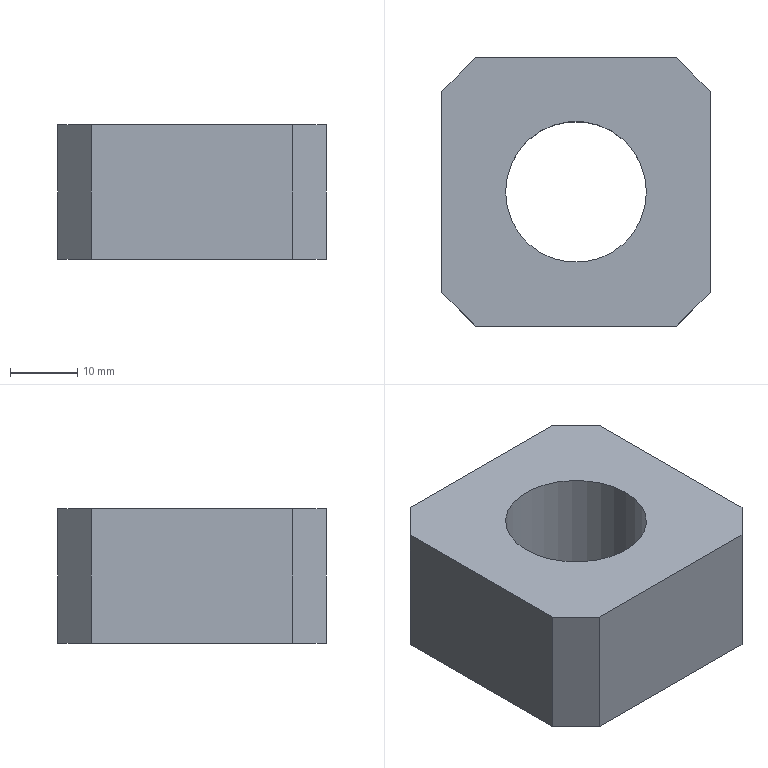NC program | NX | posted with a generic post | part box 40 x 40 x 20 mm
Whole program:
N10 G17 G21 G94 G90
(ADAPTIVE_MILLING_COPY_1 , TOOL : D10开粗)
N12 T05 M6
N14 G54
N16 G17 G0 G90 X-33.049 Y-20.536 S3500 M3
N18 G43 Z30. H5
N20 Z3.1
N22 G94 G1 X-32.899 Y-20.542 Z2.163 F1500.
N24 X-32.749 Y-20.549 Z1.792
N26 X-32.599 Y-20.555 Z1.52
N28 X-32.449 Y-20.561 Z1.3
N30 X-32.3 Y-20.568 Z1.116
N32 X-32.15 Y-20.574 Z0.958
N34 X-32. Y-20.581 Z0.82
N36 X-31.85 Y-20.587 Z0.7
N38 X-31.7 Y-20.593 Z0.595
N40 X-31.55 Y-20.6 Z0.502
N42 X-31.4 Y-20.606 Z0.421
N44 X-31.251 Y-20.613 Z0.35
N46 X-31.101 Y-20.619 Z0.29
N48 X-30.951 Y-20.625 Z0.238
N50 X-30.801 Y-20.632 Z0.195
N52 X-30.651 Y-20.638 Z0.161
N54 X-30.501 Y-20.645 Z0.134
N56 X-30.351 Y-20.651 Z0.115
N58 X-30.202 Y-20.657 Z0.104
N60 X-30.052 Y-20.664 Z0.1
N62 X-28.523 Y-20.729
N64 G3 X-27.505 Y-19.981 R1.01
N66 X-27.242 Y-16.948 R15.515
N68 X-27.2 Y-10.244 R592.762
N70 G1 X-27.198 Y20.693
N72 G2 X-24.571 Y25.413 R5.737
N74 X-20.324 Y26.917 R9.801
N76 X-14.522 Y27.19 R46.809
N78 G1 X-9.309 Y27.2
N80 X20.692 Y27.198
N82 G2 X25.369 Y24.633 R5.722
N84 X26.9 Y20.444 R9.633
N86 X27.187 Y14.906 R42.38
N88 G1 X27.2 Y9.281
N90 X27.198 Y-20.679
N92 G2 X24.594 Y-25.392 R5.737
N94 X20.28 Y-26.922 R9.807
N96 X14.44 Y-27.19 R47.799
N98 G1 X8.928 Y-27.2
N100 X-20.604 Y-27.199
N102 G2 X-25.345 Y-24.661 R5.722
N104 X-26.773 Y-20.525 R8.599
N106 X-26.912 Y-16.142 R43.012
N108 G1 X-26.9 Y-8.932
N110 X-26.899 Y19.193
N112 G2 X-23.364 Y25.142 R6.971
N114 X-18.636 Y26.621 R11.938
N116 X-12.533 Y26.888 R55.522
N118 G1 X-6.72 Y26.9
N120 X19.192 Y26.898
N122 G2 X25.165 Y23.325 R6.978
N124 X26.63 Y18.556 R12.069
N126 X26.888 Y12.64 R55.725
N128 G1 X26.899 Y7.278
N130 X26.898 Y-19.217
N132 G2 X23.336 Y-25.156 R6.98
N134 X18.604 Y-26.624 R12.015
N136 X12.35 Y-26.89 R57.25
N138 G1 X6.575 Y-26.9
N140 X-19.217 Y-26.898
N142 G2 X-25.194 Y-23.143 R6.82
N144 X-26.439 Y-18.463 R12.117
N146 X-26.598 Y-12.73 R71.518
N148 G1 X-26.6 Y-10.255
N150 X-26.598 Y17.808
N152 G2 X-22.197 Y24.971 R7.868
N154 X-17.27 Y26.331 R13.908
N156 X-10.941 Y26.588 R64.101
N158 G1 X-5.991 Y26.599
N160 X17.804 Y26.597
N162 G2 X24.955 Y22.227 R7.863
N164 X26.34 Y17.193 R13.966
N166 X26.592 Y10.113 R73.066
N168 G1 X26.599 Y5.988
N170 X26.598 Y-17.791
N172 G2 X22.197 Y-24.969 R7.872
N174 X17.31 Y-26.326 R13.869
N176 X10.718 Y-26.589 R65.387
N178 G1 X4.943 Y-26.599
N180 X-17.792 Y-26.598
N182 G2 X-24.818 Y-22.247 R7.64
N184 X-26.091 Y-17.376 R13.614
N186 X-26.294 Y-11.044 R72.736
N188 G1 X-26.3 Y-6.507
N190 X-26.298 Y16.567
N192 G2 X-24.928 Y21.595 R8.969
N194 X-20.056 Y25.221 R9.364
N196 X-14.753 Y26.151 R20.
N198 X-6.73 Y26.297 R146.883
N200 G1 X16.267 Y26.299
N202 G2 X20.613 Y25.476 R9.774
N204 X24.987 Y20.672 R8.891
N206 X26.109 Y15.335 R17.659
N208 X26.297 Y6.901 R121.733
N210 G1 X26.299 Y3.601
N212 X26.297 Y-16.555
N214 G2 X24.914 Y-21.615 R8.972
N216 X20.077 Y-25.212 R9.365
N218 X14.626 Y-26.158 R20.195
N220 X5.403 Y-26.298 R177.641
N222 G1 X-16.254 Y-26.299
N224 G2 X-20.559 Y-25.47 R9.497
N226 X-24.816 Y-20.672 R8.705
N228 X-25.844 Y-15.465 R17.595
N230 X-25.997 Y-8.193 R119.783
N232 G1 X-26. Y-4.48
N234 X-25.998 Y15.329
N236 G2 X-25.204 Y19.8 R10.961
N238 X-20.275 Y24.529 R9.234
N240 X-14.924 Y25.759 R17.439
N242 X-7.055 Y25.993 R95.576
N244 G1 X-2.105 Y25.999
N246 X15.254 Y25.998
N248 G2 X19.628 Y25.276 R11.231
N250 X24.518 Y20.302 R9.202
N252 X25.749 Y15.028 R17.246
N254 X25.994 Y6.972 R94.179
N256 G1 X25.999 Y2.435
N258 X25.997 Y-15.391
N260 G2 X25.163 Y-19.891 R10.767
N262 X20.219 Y-24.552 R9.27
N264 X14.939 Y-25.757 R17.515
N266 X6.845 Y-25.994 R97.367
N268 G1 X2.308 Y-25.999
N270 X-15.392 Y-25.997
N272 G2 X-19.916 Y-25.11 R10.327
N274 X-24.358 Y-20.239 R9.109
N276 X-25.504 Y-14.87 R17.702
N278 X-25.696 Y-7.074 R109.534
N280 G1 X-25.699 Y-2.949
N282 X-25.698 Y14.204
N284 G2 X-25.118 Y18.532 R13.216
N286 X-19.915 Y24.078 R9.477
N288 X-14.398 Y25.423 R17.467
N290 X-6.98 Y25.689 R83.266
N292 G1 X-1.205 Y25.698
N294 X14.242 Y25.697
N296 G2 X18.603 Y25.093 R13.026
N298 X24.065 Y19.942 R9.475
N300 X25.408 Y14.542 R17.238
N302 X25.689 Y6.937 R81.095
N304 G1 X25.698 Y1.162
N306 X25.697 Y-14.229
N308 G2 X25.096 Y-18.591 R13.073
N310 X19.967 Y-24.052 R9.468
N312 X14.344 Y-25.427 R17.479
N314 X6.964 Y-25.689 R84.191
N316 G1 X1.189 Y-25.698
N318 X-14.229 Y-25.697
N320 G2 X-18.514 Y-25.09 R12.561
N322 X-23.834 Y-20.017 R9.295
N324 X-25.148 Y-14.536 R17.186
N326 X-25.391 Y-7.155 R86.685
N328 G1 X-25.399 Y-1.792
N330 X-25.398 Y13.117
N332 G2 X-24.954 Y17.393 R16.031
N334 X-19.52 Y23.659 R9.748
N336 X-13.949 Y25.083 R17.521
N338 X-6.608 Y25.384 R75.983
N340 G1 X-0.008 Y25.398
N342 X13.154 Y25.397
N344 G2 X17.537 Y24.913 R15.59
N346 X23.632 Y19.576 R9.74
N348 X25.076 Y14.012 R17.369
N350 X25.387 Y6.146 R79.024
N352 G1 X25.398 Y-0.041
N354 X25.397 Y-13.142
N356 G2 X24.916 Y-17.525 R15.64
N358 X19.439 Y-23.695 R9.776
N360 X13.75 Y-25.104 R17.916
N362 X5.996 Y-25.388 R84.539
N364 G1 X0.221 Y-25.398
N366 X-13.104 Y-25.397
N368 G2 X-17.376 Y-24.928 R15.231
N370 X-23.41 Y-19.612 R9.58
N372 X-24.814 Y-13.999 R17.389
N374 X-25.089 Y-6.507 R81.982
N376 G1 X-25.099 Y-0.732
N378 X-25.098 Y12.067
N380 G2 X-24.727 Y16.428 R19.116
N382 X-19.044 Y23.294 R10.041
N384 X-13.405 Y24.758 R17.875
N386 X-6.066 Y25.081 R73.481
N388 G1 X0.947 Y25.098
N390 G2 X13.566 Y25.073 R883.653
N392 X18.614 Y23.948 R12.059
N394 X23.491 Y18.605 R10.333
N396 X24.816 Y12.854 R19.332
N398 X25.091 Y4.386 R97.895
N400 G1 X25.098 Y-0.976
N402 G2 X25.072 Y-13.591 R877.786
N404 X23.936 Y-18.636 R12.001
N406 X18.456 Y-23.552 R10.383
N408 X12.768 Y-24.824 R19.72
N410 X4.263 Y-25.091 R100.704
N412 G1 X-1.1 Y-25.098
N414 G2 X-13.516 Y-25.073 R869.408
N416 X-18.589 Y-23.888 R11.641
N418 X-23.333 Y-18.454 R10.277
N420 X-24.561 Y-12.678 R20.017
N422 X-24.791 Y-4.996 R102.276
N424 G1 X-24.799 Y0.367
N426 G2 X-24.766 Y12.966 R695.277
N428 X-23.623 Y18.088 R12.565
N430 X-18.063 Y23.168 R10.611
N432 X-12.2 Y24.508 R19.972
N434 X-3.47 Y24.79 R100.959
N436 G1 X1.892 Y24.798
N438 G2 X12.966 Y24.765 R584.678
N440 X18.19 Y23.571 R12.491
N442 X23.199 Y17.987 R10.652
N444 X24.523 Y12.044 R20.323
N446 X24.79 Y3.463 R103.915
N448 G1 X24.798 Y-1.899
N450 G2 X24.763 Y-13.029 R530.358
N452 X23.526 Y-18.278 R12.338
N454 X17.981 Y-23.201 R10.672
N456 X12.034 Y-24.523 R20.358
N458 X3.379 Y-24.791 R104.815
N460 G1 X-1.984 Y-24.798
N462 G2 X-12.954 Y-24.762 R509.573
N464 X-18.162 Y-23.504 R12.012
N466 X-22.959 Y-18.016 R10.553
N468 X-24.237 Y-12.176 R20.208
N470 X-24.49 Y-4.082 R101.04
N472 G1 X-24.498 Y1.28
N474 G2 X-24.462 Y12.291 R531.23
N476 X-23.338 Y17.496 R13.21
N478 X-17.629 Y22.809 R10.831
N480 X-11.734 Y24.185 R20.152
N482 X-3.68 Y24.485 R90.169
N484 G1 X2.507 Y24.497
N486 G2 X12.291 Y24.462 R456.381
N488 X17.428 Y23.369 R13.265
N490 X22.779 Y17.697 R10.805
N492 X24.196 Y11.621 R20.222
N494 X24.489 Y2.854 R99.947
N496 G1 X24.497 Y-2.508
N498 G2 X24.461 Y-12.316 R441.93
N500 X23.31 Y-17.553 R13.133
N502 X17.678 Y-22.786 R10.826
N504 X11.751 Y-24.182 R20.063
N506 X3.697 Y-24.485 R89.522
N508 G1 X-2.49 Y-24.497
N510 G2 X-12.241 Y-24.46 R419.199
N512 X-17.4 Y-23.305 R12.805
N514 X-22.545 Y-17.7 R10.717
N516 X-23.904 Y-11.798 R20.059
N518 X-24.186 Y-3.893 R91.732
N520 G1 X-24.198 Y2.295
N522 G2 X-24.16 Y11.616 R416.028
N524 X-23.091 Y16.837 R13.964
N526 X-17.27 Y22.426 R11.007
N528 X-11.348 Y23.855 R20.146
N530 X-3.108 Y24.183 R86.996
N532 X11.391 Y24.168 R853.682
N534 X16.457 Y23.25 R14.718
N536 X22.386 Y17.358 R10.946
N538 X23.849 Y11.408 R19.914
N540 X24.183 Y3.093 R86.191
N542 X24.167 Y-11.417 R818.503
N544 X23.198 Y-16.584 R14.524
N546 X17.361 Y-22.384 R10.954
N548 X11.408 Y-23.848 R19.916
N550 X3.093 Y-24.183 R86.009
N552 X-11.267 Y-24.169 R856.595
N554 X-16.397 Y-23.206 R14.303
N556 X-22.107 Y-17.456 R10.827
N558 X-23.558 Y-11.544 R19.672
N560 X-23.885 Y-3.304 R85.969
N562 X-23.865 Y10.791 R736.974
N564 X-22.945 Y15.933 R15.294
N566 X-16.948 Y22.033 R11.147
N568 X-11.006 Y23.522 R20.033
N570 X-3.03 Y23.877 R80.099
N572 X10.716 Y23.866 R727.505
N574 X15.795 Y22.997 R15.594
N576 X22.005 Y17.007 R11.119
N578 X23.54 Y10.846 R20.159
N580 X23.881 Y2.494 R86.621
N582 X23.867 Y-10.704 R733.224
N584 X23.002 Y-15.782 R15.629
N586 X17.017 Y-21.999 R11.117
N588 X10.894 Y-23.534 R20.093
N590 X2.917 Y-23.878 R82.261
N592 X-10.704 Y-23.863 R627.522
N594 X-15.873 Y-22.898 R14.792
N596 X-21.763 Y-17.012 R11.042
N598 X-23.243 Y-11.029 R19.998
N600 X-23.58 Y-3.089 R82.366
N602 X-23.563 Y10.154 R617.82
N604 X-22.67 Y15.341 R16.043
N606 X-16.632 Y21.642 R11.305
N608 X-10.441 Y23.216 R20.237
N610 X-2.465 Y23.575 R80.806
N612 X10.229 Y23.559 R518.663
N614 X15.411 Y22.643 R15.819
N616 X21.654 Y16.606 R11.313
N618 X23.223 Y10.378 R20.36
N620 X23.581 Y1.801 R86.775
N622 X23.557 Y-10.286 R481.157
N624 X22.622 Y-15.464 R15.655
N626 X16.488 Y-21.705 R11.35
N628 X10.283 Y-23.233 R20.696
N630 X1.594 Y-23.582 R89.777
N632 X-10.216 Y-23.555 R445.298
N634 X-15.455 Y-22.553 R15.064
N636 X-21.449 Y-16.518 R11.267
N638 X-22.94 Y-10.42 R20.549
N640 X-23.278 Y-2.518 R83.303
N642 X-23.258 Y9.629 R482.682
N644 X-22.321 Y14.959 R16.335
N646 X-16.116 Y21.349 R11.517
N648 X-9.883 Y22.912 R20.763
N650 X-1.157 Y23.28 R87.456
N652 X9.829 Y23.249 R357.735
N654 X15.181 Y22.232 R15.726
N656 X21.356 Y16.099 R11.535
N658 X22.926 Y9.754 R20.99
N660 X23.276 Y1.664 R84.983
N662 X23.257 Y-9.623 R430.442
N664 X22.322 Y-14.953 R16.351
N666 X16.082 Y-21.362 R11.527
N668 X9.847 Y-22.915 R20.889
N670 X1.759 Y-23.275 R82.927
N672 X-9.641 Y-23.252 R377.735
N674 X-14.923 Y-22.26 R15.615
N676 X-21.079 Y-16.165 R11.431
N678 X-22.635 Y-9.855 R20.824
N680 X-22.982 Y-1.203 R90.155
N682 X-22.942 Y9.371 R307.167
N684 X-21.889 Y14.792 R15.933
N686 X-15.703 Y21.014 R11.708
N688 X-9.511 Y22.588 R20.874
N690 X-1.424 Y22.971 R79.645
N692 X9.226 Y22.948 R318.405
N694 X14.587 Y21.971 R16.422
N696 X21.02 Y15.688 R11.697
N698 X22.589 Y9.495 R20.926
N700 X22.973 Y1.22 R81.362
N702 X22.944 Y-9.317 R297.003
N704 X21.909 Y-14.741 R16.087
N706 X15.689 Y-21.018 R11.71
N708 X9.42 Y-22.597 R21.052
N710 X1.033 Y-22.975 R83.542
N712 X-9.092 Y-22.948 R304.903
N714 X-14.448 Y-21.949 R16.068
N716 X-20.733 Y-15.768 R11.599
N718 X-22.317 Y-9.424 R20.982
N720 X-22.674 Y-1.41 R83.194
N722 X-22.641 Y8.789 R273.614
N724 X-21.597 Y14.288 R16.504
N726 X-15.26 Y20.697 R11.878
N728 X-8.918 Y22.291 R21.352
N730 X-0.53 Y22.673 R83.954
N732 X8.994 Y22.63 R215.903
N734 X14.514 Y21.502 R15.914
N736 X20.696 Y15.259 R11.895
N738 X22.29 Y8.92 R21.341
N740 X22.674 Y0.457 R84.392
N742 X22.632 Y-8.954 R220.738
N744 X21.547 Y-14.406 R16.095
N746 X15.184 Y-20.728 R11.906
N748 X8.875 Y-22.295 R21.544
N750 X0.375 Y-22.674 R85.473
N752 X-8.774 Y-22.633 R215.99
N754 X-14.329 Y-21.495 R15.763
N756 X-20.406 Y-15.34 R11.797
N758 X-22.008 Y-8.925 R21.307
N760 X-22.38 Y-0.049 R89.946
N762 X-22.331 Y8.387 R197.247
N764 X-21.268 Y13.883 R16.647
N766 X-14.955 Y20.321 R12.008
N768 X-8.515 Y21.973 R21.377
N770 X-0.128 Y22.37 R82.263
N772 X8.533 Y22.322 R176.542
N774 X14.157 Y21.153 R16.098
N776 X20.359 Y14.871 R12.05
N778 X21.988 Y8.386 R21.676
N780 X22.374 Y-0.227 R86.61
N782 X22.325 Y-8.476 R175.101
N784 X21.189 Y-14.07 R16.278
N786 X14.904 Y-20.342 R12.035
N788 X8.606 Y-21.961 R21.346
N790 X-0.155 Y-22.373 R83.199
N792 X-8.404 Y-22.321 R164.677
N794 X-13.919 Y-21.166 R15.881
N796 X-20.103 Y-14.87 R11.975
N798 X-21.694 Y-8.486 R21.626
N800 X-22.074 Y-0.06 R85.187
N802 X-22.015 Y8.113 R154.255
N804 X-20.835 Y13.736 R16.335
N806 X-14.418 Y20.055 R12.211
N808 X-7.931 Y21.678 R21.999
N810 X0.569 Y22.071 R85.352
N812 X8.255 Y22.005 R131.158
N814 X13.935 Y20.746 R15.919
N816 X20.047 Y14.435 R12.225
N818 X21.676 Y7.949 R21.953
N820 X22.069 Y-0.363 R83.616
N822 X22.008 Y-8.199 R136.763
N824 X20.752 Y-13.922 R16.023
N826 X14.329 Y-20.092 R12.252
N828 X7.907 Y-21.68 R22.184
N830 X-0.593 Y-22.071 R85.666
N832 X-8.241 Y-21.995 R118.269
N834 X-13.969 Y-20.631 R15.29
N836 X-19.84 Y-14.317 R12.216
N838 X-21.387 Y-8. R22.149
N840 X-21.77 Y0.238 R83.882
N842 X-21.683 Y8.036 R112.36
N844 X-20.3 Y13.798 R15.637
N846 X-13.918 Y19.774 R12.421
N848 X-7.273 Y21.393 R22.709
N850 X1.153 Y21.77 R88.613
N852 X8.312 Y21.661 R88.841
N854 X14.246 Y20.072 R14.939
N856 X19.878 Y13.673 R12.559
N858 X21.421 Y7.011 R23.471
N860 X21.778 Y-2.053 R99.447
N862 X21.638 Y-8.574 R72.309
N864 X19.889 Y-14.576 R14.452
N866 X13.611 Y-19.902 R12.632
N868 X6.945 Y-21.427 R23.722
N870 X-2.12 Y-21.778 R100.802
N872 X-8.565 Y-21.622 R65.518
N874 X-14.695 Y-19.683 R13.929
N876 X-19.706 Y-13.452 R12.692
N878 X-21.155 Y-6.805 R24.306
N880 X-21.483 Y2.861 R111.929
N882 X-21.233 Y9.001 R47.272
N884 X-18.672 Y15.525 R13.326
N886 X-12.483 Y19.864 R13.38
N888 X-5.731 Y21.191 R26.616
N890 X7.236 Y21.397 R121.059
N892 X13.035 Y20.145 R16.644
N894 X19.43 Y13.568 R12.504
N896 X21.069 Y6.969 R22.647
N898 X21.47 Y-1.868 R88.433
N900 X21.308 Y-8.35 R62.916
N902 X19.364 Y-14.521 R14.253
N904 X13.041 Y-19.65 R12.886
N906 X6.474 Y-21.121 R24.301
N908 X-3.004 Y-21.477 R103.391
N910 X-8.992 Y-21.206 R42.416
N912 X-15.759 Y-18.287 R12.932
N914 X-19.742 Y-12.058 R13.701
N916 X-20.933 Y-5.354 R28.459
N918 X-21.092 Y6.789 R116.291
N920 X-19.818 Y12.658 R16.86
N922 X-13.35 Y19.03 R12.588
N924 X-6.731 Y20.737 R22.317
N926 X2.18 Y21.166 R84.155
N928 X8.359 Y20.948 R49.475
N930 X14.815 Y18.589 R13.759
N932 X19.454 Y12.33 R13.299
N934 X20.857 Y5.595 R25.803
N936 X21.071 Y-7.07 R101.179
N938 X19.7 Y-12.914 R16.218
N940 X13.125 Y-19.129 R12.67
N942 X6.523 Y-20.76 R22.979
N944 X-2.576 Y-21.168 R88.621
N946 X-8.527 Y-20.899 R41.802
N948 X-15.276 Y-18.048 R13.144
N950 X-19.396 Y-11.736 R13.745
N952 X-20.628 Y-4.889 R28.542
N954 X-20.769 Y6.579 R98.568
N956 X-19.362 Y12.566 R16.468
N958 X-12.881 Y18.746 R12.756
N960 X-6.219 Y20.438 R22.758
N962 X6.739 Y20.754 R86.196
N964 X12.745 Y19.274 R16.078
N966 X18.792 Y12.775 R12.803
N968 X20.452 Y6.103 R23.083
N970 X20.756 Y-6.706 R87.086
N972 X19.335 Y-12.617 R16.225
N974 X12.824 Y-18.769 R12.781
N976 X6.156 Y-20.445 R22.955
N978 X-6.466 Y-20.76 R85.419
N980 X-12.341 Y-19.358 R16.149
N982 X-18.535 Y-12.755 R12.737
N984 X-20.155 Y-6.19 R23.066
N986 X-20.442 Y6.394 R81.827
N988 X-18.938 Y12.395 R16.146
N990 X-12.435 Y18.453 R12.908
N992 X-5.88 Y20.12 R22.926
N994 X6.327 Y20.443 R77.398
N996 X12.335 Y18.966 R16.246
N998 X18.454 Y12.431 R12.904
N1000 X20.147 Y5.653 R23.252
N1002 X20.433 Y-6.444 R76.598
N1004 X18.878 Y-12.508 R15.956
N1006 X12.326 Y-18.498 R12.953
N1008 X5.534 Y-20.16 R23.613
N1010 X-6.263 Y-20.432 R74.79
N1012 X-12.286 Y-18.874 R15.778
N1014 X-18.204 Y-12.392 R12.881
N1016 X-19.831 Y-5.901 R23.044
N1018 X-20.119 Y6.118 R71.971
N1020 X-18.521 Y12.208 R15.972
N1022 X-11.969 Y18.171 R13.064
N1024 X-5.258 Y19.837 R23.542
N1026 X5.975 Y20.125 R69.313
N1028 X12.013 Y18.616 R16.26
N1030 X18.185 Y11.934 R13.048
N1032 X19.832 Y5.295 R23.545
N1034 X20.113 Y-6.125 R68.036
N1036 X18.495 Y-12.252 R15.891
N1038 X11.833 Y-18.227 R13.118
N1040 X5.113 Y-19.852 R23.98
N1042 X-5.822 Y-20.121 R67.374
N1044 X-11.986 Y-18.511 R15.877
N1046 X-17.9 Y-11.971 R13.013
N1048 X-19.557 Y-5.181 R23.719
N1050 X-19.803 Y5.753 R64.867
N1052 X-18.126 Y11.974 R15.923
N1054 X-11.589 Y17.852 R13.188
N1056 X-4.73 Y19.542 R23.871
N1058 X5.903 Y19.783 R60.153
N1060 X12.141 Y18.033 R15.631
N1062 X17.889 Y11.504 R13.229
N1064 X19.54 Y4.746 R24.
N1066 X19.784 Y-5.887 R60.254
N1068 X18.076 Y-12.06 R15.69
N1070 X11.509 Y-17.885 R13.218
N1072 X4.793 Y-19.534 R23.941
N1074 X-5.541 Y-19.795 R59.671
N1076 X-11.725 Y-18.128 R15.755
N1078 X-17.564 Y-11.629 R13.119
N1080 X-19.249 Y-4.769 R23.828
N1082 X-19.479 Y5.453 R57.864
N1084 X-17.754 Y11.697 R15.86
N1086 X-11.194 Y17.543 R13.305
N1088 X-4.448 Y19.22 R23.889
N1090 X5.622 Y19.456 R53.667
N1092 X11.915 Y17.632 R15.506
N1094 X17.609 Y11.039 R13.374
N1096 X19.239 Y4.281 R24.388
N1098 X19.464 Y-5.528 R54.208
N1100 X17.677 Y-11.832 R15.637
N1102 X11.008 Y-17.62 R13.378
N1104 X4.022 Y-19.267 R24.856
N1106 X-5.525 Y-19.443 R51.512
N1108 X-11.958 Y-17.463 R15.087
N1110 X-17.392 Y-10.906 R13.426
N1112 X-18.963 Y-4.171 R24.843
N1114 X-19.143 Y5.264 R51.075
N1116 X-17.215 Y11.718 R15.484
N1118 X-10.71 Y17.274 R13.49
N1120 X-3.731 Y18.949 R24.684
N1122 X5.478 Y19.113 R47.245
N1124 X11.903 Y17.102 R15.153
N1126 X17.314 Y10.613 R13.543
N1128 X18.96 Y3.625 R24.985
N1130 X19.109 Y-5.51 R47.026
N1132 X17.062 Y-11.965 R15.071
N1134 X10.485 Y-17.365 R13.6
N1136 X3.524 Y-18.97 R25.371
N1138 X-5.236 Y-19.113 R45.961
N1140 X-11.754 Y-17.041 R14.976
N1142 X-17.062 Y-10.561 R13.543
N1144 X-18.672 Y-3.605 R25.162
N1146 X-18.791 Y5.192 R44.646
N1148 X-16.624 Y11.794 R15.033
N1150 X-9.968 Y17.11 R13.795
N1152 X-2.924 Y18.684 R26.031
N1154 X5.275 Y18.772 R41.696
N1156 X12.001 Y16.486 R14.821
N1158 X17.111 Y9.964 R13.823
N1160 X18.673 Y3.03 R25.873
N1162 X18.762 Y-5.355 R41.447
N1164 X16.402 Y-12.124 R14.699
N1166 X9.84 Y-17.158 R13.905
N1168 X2.977 Y-18.677 R26.165
N1170 X-5.258 Y-18.745 R39.736
N1172 X-12.027 Y-16.294 R14.434
N1174 X-16.932 Y-9.715 R13.959
N1176 X-18.421 Y-2.614 R26.96
N1178 X-18.403 Y5.358 R37.688
N1180 X-15.672 Y12.335 R14.313
N1182 X-9.2 Y16.948 R14.266
N1184 X-1.945 Y18.429 R27.626
N1186 X5.54 Y18.367 R34.791
N1188 X12.653 Y15.416 R14.058
N1190 X17.076 Y8.844 R14.528
N1192 X18.474 Y1.38 R29.225
N1194 X18.317 Y-5.878 R32.769
N1196 X14.804 Y-13.346 R13.707
N1198 X8.19 Y-17.291 R15.173
N1200 X0.544 Y-18.524 R31.814
N1202 X-6.147 Y-18.228 R28.797
N1204 X-16.149 Y-10.458 R13.299
N1206 X-17.958 Y-3.634 R23.17
N1208 X-18.09 Y4.895 R36.024
N1210 X-15.406 Y11.904 R14.419
N1212 X-8.901 Y16.608 R14.289
N1214 X-1.652 Y18.108 R27.196
N1216 X5.604 Y17.975 R30.623
N1218 X13.287 Y14.198 R13.64
N1220 X17.01 Y7.719 R15.455
N1222 X18.232 Y-0.417 R32.183
N1224 X17.707 Y-6.938 R24.164
N1226 X10.166 Y-16.071 R13.353
N1228 X3.237 Y-17.938 R23.101
N1230 X-4.842 Y-18.048 R32.941
N1232 X-11.96 Y-15.157 R14.053
N1234 X-16.407 Y-8.688 R14.44
N1236 X-17.858 Y-1.011 R28.219
N1238 X-17.54 Y5.9 R26.923
N1240 X-9.791 Y15.764 R13.462
N1242 X-2.752 Y17.641 R23.22
N1244 X5.174 Y17.655 R29.891
N1246 X12.933 Y13.88 R13.685
N1248 X16.697 Y7.348 R15.514
N1250 X17.71 Y-4.793 R31.374
N1252 X14.63 Y-12.112 R14.04
N1254 X8.091 Y-16.452 R14.731
N1256 X-0.159 Y-17.872 R28.961
N1258 X-6.816 Y-17.25 R21.852
N1260 X-15.436 Y-9.898 R13.315
N1262 X-17.338 Y-2.825 R22.901
N1264 X-17.322 Y4.914 R28.614
N1266 X-13.186 Y12.948 R13.652
N1268 X-6.626 Y16.49 R16.01
N1270 X4.595 Y17.352 R29.14
N1272 X12.267 Y13.862 R13.836
N1274 X16.272 Y7.335 R15.212
N1276 X17.345 Y-4.641 R28.871
N1278 X13.746 Y-12.389 R13.79
N1280 X7.15 Y-16.329 R15.36
N1282 X-4.497 Y-17.325 R28.167
N1284 X-12.393 Y-13.483 R13.607
N1286 X-16.154 Y-6.803 R15.668
N1288 X-17.013 Y4.375 R27.978
N1290 X-13.198 Y12.28 R13.755
N1292 X-6.574 Y16.085 R15.662
N1294 X4.486 Y16.976 R26.845
N1296 X12.811 Y12.629 R13.572
N1298 X16.283 Y5.874 R16.405
N1300 X16.974 Y-4.5 R26.869
N1302 X12.586 Y-12.847 R13.56
N1304 X5.889 Y-16.277 R16.414
N1306 X-4.223 Y-16.971 R26.273
N1308 X-12.613 Y-12.548 R13.478
N1310 X-16.012 Y-5.817 R16.44
N1312 X-16.624 Y4.336 R25.796
N1314 X-8.798 Y14.778 R13.562
N1316 X-1.015 Y16.739 R22.764
N1318 X6.128 Y16.213 R20.366
N1320 X14.693 Y8.969 R13.428
N1322 X16.7 Y1.43 R22.285
N1324 X16.282 Y-5.871 R20.994
N1326 X8.986 Y-14.682 R13.424
N1328 X1.15 Y-16.718 R22.309
N1330 X-5.954 Y-16.185 R19.86
N1332 X-14.37 Y-9.059 R13.34
N1334 X-16.403 Y-1.336 R21.98
N1336 X-15.874 Y5.842 R19.982
N1338 X-8.53 Y14.42 R13.491
N1340 X0.07 Y16.439 R22.351
N1342 X6.971 Y15.486 R17.513
N1344 X14.407 Y8.552 R13.472
N1346 X16.436 Y-0.005 R22.28
N1348 X15.494 Y-6.946 R17.564
N1350 X8.485 Y-14.436 R13.486
N1352 X-0.831 Y-16.439 R22.303
N1354 X-7.959 Y-14.942 R15.793
N1356 X-14.242 Y-8.307 R13.582
N1358 X-15.843 Y4.129 R22.059
N1360 X-8.195 Y14.094 R13.498
N1362 X4.22 Y15.798 R21.329
N1364 X14.043 Y8.294 R13.419
N1366 X15.798 Y-4.218 R21.293
N1368 X8.324 Y-14.025 R13.411
N1370 X-4.034 Y-15.772 R20.819
N1372 X-13.723 Y-8.37 R13.326
N1374 X-15.435 Y4.063 R20.61
N1376 X-7.99 Y13.704 R13.424
N1378 X4.111 Y15.395 R20.011
N1380 X13.676 Y8.039 R13.351
N1382 X15.397 Y-4.094 R19.991
N1384 X8.005 Y-13.691 R13.356
N1386 X-3.836 Y-15.382 R19.596
N1388 X-13.33 Y-8.165 R13.244
N1390 X-15.049 Y3.845 R19.411
N1392 X-7.7 Y13.355 R13.353
N1394 X3.953 Y14.992 R18.831
N1396 X13.331 Y7.738 R13.273
N1398 X14.993 Y-3.947 R18.81
N1400 X7.768 Y-13.313 R13.263
N1402 X-3.659 Y-14.981 R18.449
N1404 X-13.002 Y-7.826 R13.168
N1406 X-14.633 Y3.743 R18.258
N1408 X-7.393 Y13.012 R13.259
N1410 X3.739 Y14.595 R17.774
N1412 X12.981 Y7.445 R13.174
N1414 X14.583 Y-3.791 R17.722
N1416 X7.45 Y-12.974 R13.162
N1418 X-3.599 Y-14.549 R17.347
N1420 X-12.677 Y-7.477 R13.071
N1422 X-14.222 Y3.577 R17.225
N1424 X-7.125 Y12.647 R13.134
N1426 X3.744 Y14.143 R16.71
N1428 X12.605 Y7.193 R13.039
N1430 X14.143 Y-3.741 R16.687
N1432 X7.12 Y-12.638 R13.04
N1434 X-3.528 Y-14.109 R16.333
N1436 X-12.327 Y-7.171 R12.935
N1438 X-13.755 Y3.62 R16.198
N1440 X-6.748 Y12.333 R13.004
N1442 X3.759 Y13.677 R15.733
N1444 X12.272 Y6.854 R12.899
N1446 X13.677 Y-3.751 R15.708
N1448 X6.817 Y-12.285 R12.886
N1450 X-3.576 Y-13.63 R15.368
N1452 X-11.993 Y-6.824 R12.784
N1454 X-13.263 Y3.711 R15.241
N1456 X-6.242 Y12.077 R12.872
N1458 X3.912 Y13.161 R14.789
N1460 X11.983 Y6.416 R12.754
N1462 X13.18 Y-3.831 R14.783
N1464 X6.263 Y-12.05 R12.745
N1466 X-3.671 Y-13.123 R14.443
N1468 X-11.729 Y-6.325 R12.629
N1470 X-12.736 Y3.859 R14.334
N1472 X-5.75 Y11.803 R12.697
N1474 X4.087 Y12.616 R13.9
N1476 X11.821 Y5.692 R12.625
N1478 X12.584 Y-4.183 R13.839
N1480 X5.55 Y-11.875 R12.605
N1482 X-4.221 Y-12.453 R13.487
N1484 X-11.614 Y-5.47 R12.523
N1486 X-12.061 Y4.374 R13.391
N1488 X-4.784 Y11.716 R12.574
N1490 X5.051 Y11.743 R12.911
N1492 X11.854 Y4.405 R12.594
N1494 X11.56 Y-5.455 R12.774
N1496 X3.682 Y-12.075 R12.643
N1498 X-6.366 Y-10.891 R12.291
N1500 X-12.2 Y-1.709 R12.839
N1502 X-5.086 Y11.073 R12.039
N1504 X5.271 Y11.091 R12.297
N1506 X11.907 Y2.575 R12.42
N1508 X5.015 Y-11.075 R11.86
N1510 X-5.554 Y-10.77 R11.966
N1512 X-11.143 Y3.968 R12.254
N1514 X-1.835 Y11.566 R11.987
N1516 X10.523 Y5.081 R11.49
N1518 X9.951 Y-6.248 R11.613
N1520 X-3.381 Y-11.132 R11.779
N1522 X-11.18 Y-1.932 R11.587
N1524 X-3.768 Y10.543 R11.268
N1526 X10.314 Y4.314 R11.097
N1528 X3.413 Y-10.611 R11.052
N1530 X-10.094 Y-4. R10.858
N1532 X-1.658 Y10.553 R10.827
N1534 X10.191 Y3.126 R10.651
N1536 X-3.864 Y-9.792 R10.543
N1538 X-9.075 Y4.644 R10.432
N1540 X4.214 Y9.205 R10.231
N1542 X8.833 Y-4.917 R10.128
N1544 X-4.928 Y-8.601 R9.92
N1546 X-5.89 Y7.536 R9.793
N1548 X8.135 Y-4.928 R9.538
N1550 X-8.986 Y1.129 R9.27
N1552 X4.72 Y7.545 R9.025
N1554 X1.415 Y-8.68 R8.825
N1556 X-5.984 Y5.755 R8.559
N1558 X7.88 Y-2.255 R8.256
N1560 X-6.912 Y-3.613 R7.957
N1562 X0.687 Y7.447 R7.687
N1564 X5.055 Y-5.35 R7.408
N1566 X-6.832 Y-0.123 R7.07
N1568 X3.598 Y5.435 R6.717
N1570 X3.378 Y-5.316 R6.363
N1572 X-5.596 Y-1.03 R5.949
N1574 X-0.083 Y5.152 R5.444
N1576 X4.548 Y1.154 R4.786
N1578 X4.226 Y-1.16 R4.553
N1580 G1 X4.177 Y-1.301 Z0.104
N1582 X4.127 Y-1.443 Z0.115
N1584 X4.078 Y-1.584 Z0.134
N1586 X4.028 Y-1.726 Z0.161
N1588 X3.978 Y-1.867 Z0.195
N1590 X3.929 Y-2.009 Z0.238
N1592 X3.879 Y-2.15 Z0.29
N1594 X3.829 Y-2.292 Z0.35
N1596 X3.78 Y-2.434 Z0.421
N1598 X3.73 Y-2.575 Z0.502
N1600 X3.68 Y-2.717 Z0.595
N1602 X3.631 Y-2.858 Z0.7
N1604 X3.581 Y-3. Z0.82
N1606 X3.532 Y-3.141 Z0.958
N1608 X3.482 Y-3.283 Z1.116
N1610 X3.432 Y-3.424 Z1.3
N1612 X3.383 Y-3.566 Z1.52
N1614 X3.333 Y-3.707 Z1.792
N1616 X3.283 Y-3.849 Z2.163
N1618 X3.234 Y-3.991 Z3.1
N1620 G0 Z30.
N1622 M5
(PLANAR_MILL_COPY , TOOL : D50面刀)
N1624 T01 M6
N1626 G54
N1628 G17 G0 G90 X55. Y0. S2000 M3
N1630 G43 Z30. H1
N1632 Z2.
N1634 G94 G1 Z0. F800.
N1636 X15.
N1638 X-15.
N1640 X-55.
N1642 Z2.
N1644 G0 Z30.
N1646 M5
(PLANAR_MILL_1_COPY_COPY_1 , TOOL : D8倒角刀)
N1648 T02 M6
N1650 G54
N1652 G17 G0 G90 X-14.036 Y-24.5 S2500 M3
N1654 G43 Z30. H2
N1656 Z-0.5
N1658 G94 G1 Z-2.5 F600.
N1660 X-16.768 Y-21.767
N1662 X-21.768 Y-16.768
N1664 G2 X-22.5 Y-15. R2.5
N1666 G1 Y15.
N1668 G2 X-21.768 Y16.768 R2.5
N1670 G1 X-16.768 Y21.768
N1672 G2 X-15. Y22.5 R2.5
N1674 G1 X15.
N1676 G2 X16.768 Y21.768 R2.5
N1678 G1 X21.768 Y16.768
N1680 G2 X22.5 Y15. R2.5
N1682 G1 Y-15.
N1684 G2 X21.768 Y-16.768 R2.5
N1686 G1 X16.768 Y-21.768
N1688 G2 X15. Y-22.5 R2.5
N1690 G1 X-14.999
N1692 X-18.864
N1694 Z-0.5
N1696 G0 Z30.
(PLANAR_MILL_1_COPY_COPY_COPY , TOOL : D8倒角刀)
N1698 X6.29 Y-2. S3000
N1700 Z-0.5
N1702 G1 Z-2.5
N1704 X6.6
N1706 G3 X8.6 Y0. R2.
N1708 X0. Y8.6 R8.6
N1710 X8.6 Y0. R-8.6
N1712 X6.6 Y2. R2.
N1714 G1 X7.1 Y-2.
N1716 G3 X9.1 Y0. R2.
N1718 X0. Y9.1 R9.1
N1720 X9.1 Y0. R-9.1
N1722 X7.1 Y2. R2.
N1724 G1 X7.6 Y-2.
N1726 G3 X9.6 Y0. R2.
N1728 X0. Y9.6 R9.6
N1730 X9.6 Y0. R-9.6
N1732 X7.6 Y2. R2.
N1734 G1 X7.332
N1736 Z-0.5
N1738 G0 Z30.
N1740 M5
N1742 M2